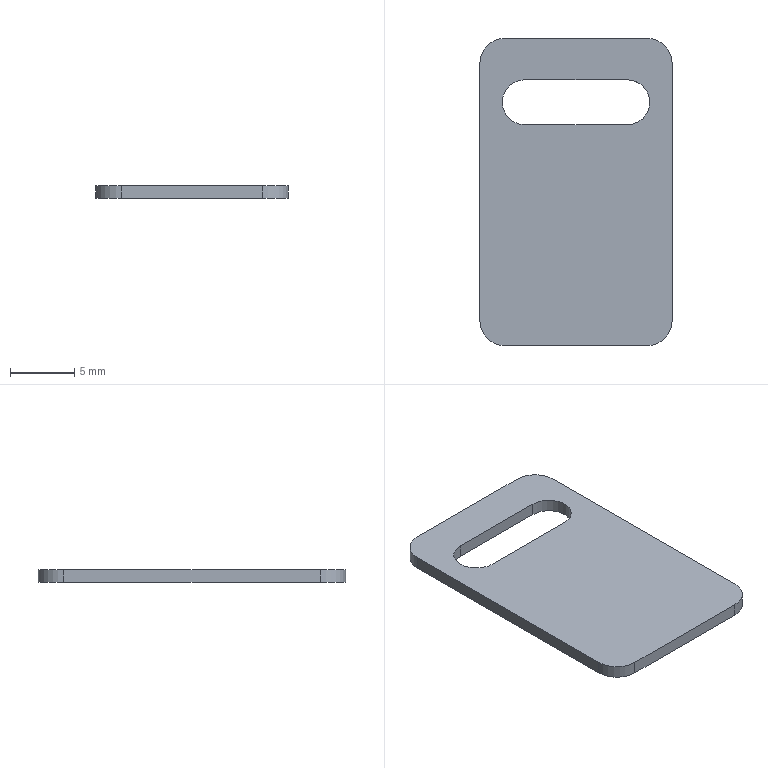Part | SolidWorks | features Extrusion 1, Fillet 1 | 1 solid | 15 faces | box 15 x 24 x 1 mm | volume 318.945 mm3 | plane 8 | cylinder 7 | commonest cylinder face diameters 4 x4 3.5 x3
STEP:
#1=CARTESIAN_POINT('',(-4.,8.75,1.));
#2=VERTEX_POINT('',#1);
#3=CARTESIAN_POINT('',(-5.75,7.,1.));
#4=VERTEX_POINT('',#3);
#5=CARTESIAN_POINT('',(-4.,7.,1.));
#6=DIRECTION('',(0.,0.,1.));
#7=DIRECTION('',(1.,0.,0.));
#8=AXIS2_PLACEMENT_3D('',#5,#6,#7);
#9=CIRCLE('',#8,1.75);
#10=EDGE_CURVE('',#2,#4,#9,.T.);
#11=ORIENTED_EDGE('',*,*,#10,.T.);
#12=CARTESIAN_POINT('',(-5.75,7.,0.));
#13=VERTEX_POINT('',#12);
#14=CARTESIAN_POINT('',(-5.75,7.,1.));
#15=DIRECTION('',(0.,0.,-1.));
#16=VECTOR('',#15,1000.);
#17=LINE('',#14,#16);
#18=EDGE_CURVE('',#4,#13,#17,.T.);
#19=ORIENTED_EDGE('',*,*,#18,.T.);
#20=CARTESIAN_POINT('',(-4.,8.75,0.));
#21=VERTEX_POINT('',#20);
#22=CARTESIAN_POINT('',(-4.,7.,0.));
#23=DIRECTION('',(0.,0.,1.));
#24=DIRECTION('',(1.,0.,0.));
#25=AXIS2_PLACEMENT_3D('',#22,#23,#24);
#26=CIRCLE('',#25,1.75);
#27=EDGE_CURVE('',#21,#13,#26,.T.);
#28=ORIENTED_EDGE('',*,*,#27,.F.);
#29=CARTESIAN_POINT('',(-4.,8.75,1.));
#30=DIRECTION('',(0.,0.,-1.));
#31=VECTOR('',#30,1000.);
#32=LINE('',#29,#31);
#33=EDGE_CURVE('',#2,#21,#32,.T.);
#34=ORIENTED_EDGE('',*,*,#33,.F.);
#35=EDGE_LOOP('',(#11,#19,#28,#34));
#36=FACE_OUTER_BOUND('',#35,.T.);
#37=CARTESIAN_POINT('',(-4.,7.,1.));
#38=DIRECTION('',(0.,0.,-1.));
#39=DIRECTION('',(-1.,0.,0.));
#40=AXIS2_PLACEMENT_3D('',#37,#38,#39);
#41=CYLINDRICAL_SURFACE('',#40,1.75);
#42=ADVANCED_FACE('',(#36),#41,.F.);
#43=CARTESIAN_POINT('',(5.5,12.,1.));
#44=VERTEX_POINT('',#43);
#45=CARTESIAN_POINT('',(-5.5,12.,1.));
#46=VERTEX_POINT('',#45);
#47=CARTESIAN_POINT('',(-7.5,12.,1.));
#48=DIRECTION('',(-1.,0.,0.));
#49=VECTOR('',#48,1000.);
#50=LINE('',#47,#49);
#51=EDGE_CURVE('',#44,#46,#50,.T.);
#52=ORIENTED_EDGE('',*,*,#51,.T.);
#53=CARTESIAN_POINT('',(-7.5,10.,1.));
#54=VERTEX_POINT('',#53);
#55=CARTESIAN_POINT('',(-5.5,10.,1.));
#56=DIRECTION('',(0.,0.,1.));
#57=DIRECTION('',(-1.,0.,0.));
#58=AXIS2_PLACEMENT_3D('',#55,#56,#57);
#59=CIRCLE('',#58,2.);
#60=EDGE_CURVE('',#46,#54,#59,.T.);
#61=ORIENTED_EDGE('',*,*,#60,.T.);
#62=CARTESIAN_POINT('',(-7.5,-10.,1.));
#63=VERTEX_POINT('',#62);
#64=CARTESIAN_POINT('',(-7.5,-12.,1.));
#65=DIRECTION('',(0.,-1.,0.));
#66=VECTOR('',#65,1000.);
#67=LINE('',#64,#66);
#68=EDGE_CURVE('',#54,#63,#67,.T.);
#69=ORIENTED_EDGE('',*,*,#68,.T.);
#70=CARTESIAN_POINT('',(-5.5,-12.,1.));
#71=VERTEX_POINT('',#70);
#72=CARTESIAN_POINT('',(-5.5,-10.,1.));
#73=DIRECTION('',(0.,0.,1.));
#74=DIRECTION('',(-1.,0.,0.));
#75=AXIS2_PLACEMENT_3D('',#72,#73,#74);
#76=CIRCLE('',#75,2.);
#77=EDGE_CURVE('',#63,#71,#76,.T.);
#78=ORIENTED_EDGE('',*,*,#77,.T.);
#79=CARTESIAN_POINT('',(5.5,-12.,1.));
#80=VERTEX_POINT('',#79);
#81=CARTESIAN_POINT('',(-7.5,-12.,1.));
#82=DIRECTION('',(1.,0.,0.));
#83=VECTOR('',#82,1000.);
#84=LINE('',#81,#83);
#85=EDGE_CURVE('',#71,#80,#84,.T.);
#86=ORIENTED_EDGE('',*,*,#85,.T.);
#87=CARTESIAN_POINT('',(7.5,-10.,1.));
#88=VERTEX_POINT('',#87);
#89=CARTESIAN_POINT('',(5.5,-10.,1.));
#90=DIRECTION('',(0.,0.,1.));
#91=DIRECTION('',(-1.,0.,0.));
#92=AXIS2_PLACEMENT_3D('',#89,#90,#91);
#93=CIRCLE('',#92,2.);
#94=EDGE_CURVE('',#80,#88,#93,.T.);
#95=ORIENTED_EDGE('',*,*,#94,.T.);
#96=CARTESIAN_POINT('',(7.5,10.,1.));
#97=VERTEX_POINT('',#96);
#98=CARTESIAN_POINT('',(7.5,-12.,1.));
#99=DIRECTION('',(0.,1.,0.));
#100=VECTOR('',#99,1000.);
#101=LINE('',#98,#100);
#102=EDGE_CURVE('',#88,#97,#101,.T.);
#103=ORIENTED_EDGE('',*,*,#102,.T.);
#104=CARTESIAN_POINT('',(5.5,10.,1.));
#105=DIRECTION('',(0.,0.,1.));
#106=DIRECTION('',(-1.,0.,0.));
#107=AXIS2_PLACEMENT_3D('',#104,#105,#106);
#108=CIRCLE('',#107,2.);
#109=EDGE_CURVE('',#97,#44,#108,.T.);
#110=ORIENTED_EDGE('',*,*,#109,.T.);
#111=EDGE_LOOP('',(#52,#61,#69,#78,#86,#95,#103,#110));
#112=FACE_OUTER_BOUND('',#111,.T.);
#113=ORIENTED_EDGE('',*,*,#10,.F.);
#114=CARTESIAN_POINT('',(4.,8.75,1.));
#115=VERTEX_POINT('',#114);
#116=CARTESIAN_POINT('',(-4.,8.75,1.));
#117=DIRECTION('',(-1.,0.,0.));
#118=VECTOR('',#117,1000.);
#119=LINE('',#116,#118);
#120=EDGE_CURVE('',#115,#2,#119,.T.);
#121=ORIENTED_EDGE('',*,*,#120,.F.);
#122=CARTESIAN_POINT('',(4.,5.25,1.));
#123=VERTEX_POINT('',#122);
#124=CARTESIAN_POINT('',(4.,7.,1.));
#125=DIRECTION('',(0.,0.,1.));
#126=DIRECTION('',(1.,0.,0.));
#127=AXIS2_PLACEMENT_3D('',#124,#125,#126);
#128=CIRCLE('',#127,1.75);
#129=EDGE_CURVE('',#123,#115,#128,.T.);
#130=ORIENTED_EDGE('',*,*,#129,.F.);
#131=CARTESIAN_POINT('',(-4.,5.25,1.));
#132=VERTEX_POINT('',#131);
#133=CARTESIAN_POINT('',(-4.,5.25,1.));
#134=DIRECTION('',(1.,0.,0.));
#135=VECTOR('',#134,1000.);
#136=LINE('',#133,#135);
#137=EDGE_CURVE('',#132,#123,#136,.T.);
#138=ORIENTED_EDGE('',*,*,#137,.F.);
#139=CARTESIAN_POINT('',(-4.,7.,1.));
#140=DIRECTION('',(0.,0.,1.));
#141=DIRECTION('',(1.,0.,0.));
#142=AXIS2_PLACEMENT_3D('',#139,#140,#141);
#143=CIRCLE('',#142,1.75);
#144=EDGE_CURVE('',#4,#132,#143,.T.);
#145=ORIENTED_EDGE('',*,*,#144,.F.);
#146=EDGE_LOOP('',(#113,#121,#130,#138,#145));
#147=FACE_BOUND('',#146,.T.);
#148=CARTESIAN_POINT('',(0.,0.,1.));
#149=DIRECTION('',(0.,0.,-1.));
#150=DIRECTION('',(-1.,0.,0.));
#151=AXIS2_PLACEMENT_3D('',#148,#149,#150);
#152=PLANE('',#151);
#153=ADVANCED_FACE('',(#112,#147),#152,.F.);
#154=CARTESIAN_POINT('',(-7.5,10.,0.));
#155=VERTEX_POINT('',#154);
#156=CARTESIAN_POINT('',(-7.5,-10.,0.));
#157=VERTEX_POINT('',#156);
#158=CARTESIAN_POINT('',(-7.5,-12.,0.));
#159=DIRECTION('',(0.,-1.,0.));
#160=VECTOR('',#159,1000.);
#161=LINE('',#158,#160);
#162=EDGE_CURVE('',#155,#157,#161,.T.);
#163=ORIENTED_EDGE('',*,*,#162,.F.);
#164=CARTESIAN_POINT('',(-5.5,12.,0.));
#165=VERTEX_POINT('',#164);
#166=CARTESIAN_POINT('',(-5.5,10.,0.));
#167=DIRECTION('',(0.,0.,-1.));
#168=DIRECTION('',(-1.,0.,0.));
#169=AXIS2_PLACEMENT_3D('',#166,#167,#168);
#170=CIRCLE('',#169,2.);
#171=EDGE_CURVE('',#155,#165,#170,.T.);
#172=ORIENTED_EDGE('',*,*,#171,.T.);
#173=CARTESIAN_POINT('',(5.5,12.,0.));
#174=VERTEX_POINT('',#173);
#175=CARTESIAN_POINT('',(-7.5,12.,0.));
#176=DIRECTION('',(-1.,0.,0.));
#177=VECTOR('',#176,1000.);
#178=LINE('',#175,#177);
#179=EDGE_CURVE('',#174,#165,#178,.T.);
#180=ORIENTED_EDGE('',*,*,#179,.F.);
#181=CARTESIAN_POINT('',(7.5,10.,0.));
#182=VERTEX_POINT('',#181);
#183=CARTESIAN_POINT('',(5.5,10.,0.));
#184=DIRECTION('',(0.,0.,-1.));
#185=DIRECTION('',(-1.,0.,0.));
#186=AXIS2_PLACEMENT_3D('',#183,#184,#185);
#187=CIRCLE('',#186,2.);
#188=EDGE_CURVE('',#174,#182,#187,.T.);
#189=ORIENTED_EDGE('',*,*,#188,.T.);
#190=CARTESIAN_POINT('',(7.5,-10.,0.));
#191=VERTEX_POINT('',#190);
#192=CARTESIAN_POINT('',(7.5,-12.,0.));
#193=DIRECTION('',(0.,1.,0.));
#194=VECTOR('',#193,1000.);
#195=LINE('',#192,#194);
#196=EDGE_CURVE('',#191,#182,#195,.T.);
#197=ORIENTED_EDGE('',*,*,#196,.F.);
#198=CARTESIAN_POINT('',(5.5,-12.,0.));
#199=VERTEX_POINT('',#198);
#200=CARTESIAN_POINT('',(5.5,-10.,0.));
#201=DIRECTION('',(0.,0.,-1.));
#202=DIRECTION('',(-1.,0.,0.));
#203=AXIS2_PLACEMENT_3D('',#200,#201,#202);
#204=CIRCLE('',#203,2.);
#205=EDGE_CURVE('',#191,#199,#204,.T.);
#206=ORIENTED_EDGE('',*,*,#205,.T.);
#207=CARTESIAN_POINT('',(-5.5,-12.,0.));
#208=VERTEX_POINT('',#207);
#209=CARTESIAN_POINT('',(-7.5,-12.,0.));
#210=DIRECTION('',(1.,0.,0.));
#211=VECTOR('',#210,1000.);
#212=LINE('',#209,#211);
#213=EDGE_CURVE('',#208,#199,#212,.T.);
#214=ORIENTED_EDGE('',*,*,#213,.F.);
#215=CARTESIAN_POINT('',(-5.5,-10.,0.));
#216=DIRECTION('',(0.,0.,-1.));
#217=DIRECTION('',(-1.,0.,0.));
#218=AXIS2_PLACEMENT_3D('',#215,#216,#217);
#219=CIRCLE('',#218,2.);
#220=EDGE_CURVE('',#208,#157,#219,.T.);
#221=ORIENTED_EDGE('',*,*,#220,.T.);
#222=EDGE_LOOP('',(#163,#172,#180,#189,#197,#206,#214,#221));
#223=FACE_OUTER_BOUND('',#222,.T.);
#224=CARTESIAN_POINT('',(4.,8.75,0.));
#225=VERTEX_POINT('',#224);
#226=CARTESIAN_POINT('',(-4.,8.75,0.));
#227=DIRECTION('',(-1.,0.,0.));
#228=VECTOR('',#227,1000.);
#229=LINE('',#226,#228);
#230=EDGE_CURVE('',#225,#21,#229,.T.);
#231=ORIENTED_EDGE('',*,*,#230,.T.);
#232=ORIENTED_EDGE('',*,*,#27,.T.);
#233=CARTESIAN_POINT('',(-4.,5.25,0.));
#234=VERTEX_POINT('',#233);
#235=CARTESIAN_POINT('',(-4.,7.,0.));
#236=DIRECTION('',(0.,0.,1.));
#237=DIRECTION('',(1.,0.,0.));
#238=AXIS2_PLACEMENT_3D('',#235,#236,#237);
#239=CIRCLE('',#238,1.75);
#240=EDGE_CURVE('',#13,#234,#239,.T.);
#241=ORIENTED_EDGE('',*,*,#240,.T.);
#242=CARTESIAN_POINT('',(4.,5.25,0.));
#243=VERTEX_POINT('',#242);
#244=CARTESIAN_POINT('',(-4.,5.25,0.));
#245=DIRECTION('',(1.,0.,0.));
#246=VECTOR('',#245,1000.);
#247=LINE('',#244,#246);
#248=EDGE_CURVE('',#234,#243,#247,.T.);
#249=ORIENTED_EDGE('',*,*,#248,.T.);
#250=CARTESIAN_POINT('',(4.,7.,0.));
#251=DIRECTION('',(0.,0.,1.));
#252=DIRECTION('',(1.,0.,0.));
#253=AXIS2_PLACEMENT_3D('',#250,#251,#252);
#254=CIRCLE('',#253,1.75);
#255=EDGE_CURVE('',#243,#225,#254,.T.);
#256=ORIENTED_EDGE('',*,*,#255,.T.);
#257=EDGE_LOOP('',(#231,#232,#241,#249,#256));
#258=FACE_BOUND('',#257,.T.);
#259=CARTESIAN_POINT('',(0.,0.,0.));
#260=DIRECTION('',(0.,0.,-1.));
#261=DIRECTION('',(-1.,0.,0.));
#262=AXIS2_PLACEMENT_3D('',#259,#260,#261);
#263=PLANE('',#262);
#264=ADVANCED_FACE('',(#223,#258),#263,.T.);
#265=ORIENTED_EDGE('',*,*,#196,.T.);
#266=CARTESIAN_POINT('',(7.5,10.,1.));
#267=DIRECTION('',(0.,0.,1.));
#268=VECTOR('',#267,1000.);
#269=LINE('',#266,#268);
#270=EDGE_CURVE('',#182,#97,#269,.T.);
#271=ORIENTED_EDGE('',*,*,#270,.T.);
#272=ORIENTED_EDGE('',*,*,#102,.F.);
#273=CARTESIAN_POINT('',(7.5,-10.,1.));
#274=DIRECTION('',(0.,0.,-1.));
#275=VECTOR('',#274,1000.);
#276=LINE('',#273,#275);
#277=EDGE_CURVE('',#88,#191,#276,.T.);
#278=ORIENTED_EDGE('',*,*,#277,.T.);
#279=EDGE_LOOP('',(#265,#271,#272,#278));
#280=FACE_OUTER_BOUND('',#279,.T.);
#281=CARTESIAN_POINT('',(7.5,-12.,1.));
#282=DIRECTION('',(-1.,0.,0.));
#283=DIRECTION('',(0.,0.,1.));
#284=AXIS2_PLACEMENT_3D('',#281,#282,#283);
#285=PLANE('',#284);
#286=ADVANCED_FACE('',(#280),#285,.F.);
#287=ORIENTED_EDGE('',*,*,#179,.T.);
#288=CARTESIAN_POINT('',(-5.5,12.,1.));
#289=DIRECTION('',(0.,0.,1.));
#290=VECTOR('',#289,1000.);
#291=LINE('',#288,#290);
#292=EDGE_CURVE('',#165,#46,#291,.T.);
#293=ORIENTED_EDGE('',*,*,#292,.T.);
#294=ORIENTED_EDGE('',*,*,#51,.F.);
#295=CARTESIAN_POINT('',(5.5,12.,1.));
#296=DIRECTION('',(0.,0.,-1.));
#297=VECTOR('',#296,1000.);
#298=LINE('',#295,#297);
#299=EDGE_CURVE('',#44,#174,#298,.T.);
#300=ORIENTED_EDGE('',*,*,#299,.T.);
#301=EDGE_LOOP('',(#287,#293,#294,#300));
#302=FACE_OUTER_BOUND('',#301,.T.);
#303=CARTESIAN_POINT('',(-7.5,12.,1.));
#304=DIRECTION('',(0.,-1.,0.));
#305=DIRECTION('',(0.,0.,-1.));
#306=AXIS2_PLACEMENT_3D('',#303,#304,#305);
#307=PLANE('',#306);
#308=ADVANCED_FACE('',(#302),#307,.F.);
#309=ORIENTED_EDGE('',*,*,#68,.F.);
#310=CARTESIAN_POINT('',(-7.5,10.,1.));
#311=DIRECTION('',(0.,0.,-1.));
#312=VECTOR('',#311,1000.);
#313=LINE('',#310,#312);
#314=EDGE_CURVE('',#54,#155,#313,.T.);
#315=ORIENTED_EDGE('',*,*,#314,.T.);
#316=ORIENTED_EDGE('',*,*,#162,.T.);
#317=CARTESIAN_POINT('',(-7.5,-10.,1.));
#318=DIRECTION('',(0.,0.,1.));
#319=VECTOR('',#318,1000.);
#320=LINE('',#317,#319);
#321=EDGE_CURVE('',#157,#63,#320,.T.);
#322=ORIENTED_EDGE('',*,*,#321,.T.);
#323=EDGE_LOOP('',(#309,#315,#316,#322));
#324=FACE_OUTER_BOUND('',#323,.T.);
#325=CARTESIAN_POINT('',(-7.5,-12.,1.));
#326=DIRECTION('',(1.,0.,0.));
#327=DIRECTION('',(0.,0.,-1.));
#328=AXIS2_PLACEMENT_3D('',#325,#326,#327);
#329=PLANE('',#328);
#330=ADVANCED_FACE('',(#324),#329,.F.);
#331=ORIENTED_EDGE('',*,*,#213,.T.);
#332=CARTESIAN_POINT('',(5.5,-12.,1.));
#333=DIRECTION('',(0.,0.,1.));
#334=VECTOR('',#333,1000.);
#335=LINE('',#332,#334);
#336=EDGE_CURVE('',#199,#80,#335,.T.);
#337=ORIENTED_EDGE('',*,*,#336,.T.);
#338=ORIENTED_EDGE('',*,*,#85,.F.);
#339=CARTESIAN_POINT('',(-5.5,-12.,1.));
#340=DIRECTION('',(0.,0.,-1.));
#341=VECTOR('',#340,1000.);
#342=LINE('',#339,#341);
#343=EDGE_CURVE('',#71,#208,#342,.T.);
#344=ORIENTED_EDGE('',*,*,#343,.T.);
#345=EDGE_LOOP('',(#331,#337,#338,#344));
#346=FACE_OUTER_BOUND('',#345,.T.);
#347=CARTESIAN_POINT('',(-7.5,-12.,1.));
#348=DIRECTION('',(0.,1.,0.));
#349=DIRECTION('',(0.,0.,1.));
#350=AXIS2_PLACEMENT_3D('',#347,#348,#349);
#351=PLANE('',#350);
#352=ADVANCED_FACE('',(#346),#351,.F.);
#353=ORIENTED_EDGE('',*,*,#18,.F.);
#354=ORIENTED_EDGE('',*,*,#144,.T.);
#355=CARTESIAN_POINT('',(-4.,5.25,1.));
#356=DIRECTION('',(0.,0.,-1.));
#357=VECTOR('',#356,1000.);
#358=LINE('',#355,#357);
#359=EDGE_CURVE('',#132,#234,#358,.T.);
#360=ORIENTED_EDGE('',*,*,#359,.T.);
#361=ORIENTED_EDGE('',*,*,#240,.F.);
#362=EDGE_LOOP('',(#353,#354,#360,#361));
#363=FACE_OUTER_BOUND('',#362,.T.);
#364=CARTESIAN_POINT('',(-4.,7.,1.));
#365=DIRECTION('',(0.,0.,-1.));
#366=DIRECTION('',(-1.,0.,0.));
#367=AXIS2_PLACEMENT_3D('',#364,#365,#366);
#368=CYLINDRICAL_SURFACE('',#367,1.75);
#369=ADVANCED_FACE('',(#363),#368,.F.);
#370=ORIENTED_EDGE('',*,*,#248,.F.);
#371=ORIENTED_EDGE('',*,*,#359,.F.);
#372=ORIENTED_EDGE('',*,*,#137,.T.);
#373=CARTESIAN_POINT('',(4.,5.25,1.));
#374=DIRECTION('',(0.,0.,-1.));
#375=VECTOR('',#374,1000.);
#376=LINE('',#373,#375);
#377=EDGE_CURVE('',#123,#243,#376,.T.);
#378=ORIENTED_EDGE('',*,*,#377,.T.);
#379=EDGE_LOOP('',(#370,#371,#372,#378));
#380=FACE_OUTER_BOUND('',#379,.T.);
#381=CARTESIAN_POINT('',(-4.,5.25,1.));
#382=DIRECTION('',(0.,1.,0.));
#383=DIRECTION('',(0.,0.,1.));
#384=AXIS2_PLACEMENT_3D('',#381,#382,#383);
#385=PLANE('',#384);
#386=ADVANCED_FACE('',(#380),#385,.T.);
#387=ORIENTED_EDGE('',*,*,#255,.F.);
#388=ORIENTED_EDGE('',*,*,#377,.F.);
#389=ORIENTED_EDGE('',*,*,#129,.T.);
#390=CARTESIAN_POINT('',(4.,8.75,1.));
#391=DIRECTION('',(0.,0.,-1.));
#392=VECTOR('',#391,1000.);
#393=LINE('',#390,#392);
#394=EDGE_CURVE('',#115,#225,#393,.T.);
#395=ORIENTED_EDGE('',*,*,#394,.T.);
#396=EDGE_LOOP('',(#387,#388,#389,#395));
#397=FACE_OUTER_BOUND('',#396,.T.);
#398=CARTESIAN_POINT('',(4.,7.,1.));
#399=DIRECTION('',(0.,0.,-1.));
#400=DIRECTION('',(-1.,0.,0.));
#401=AXIS2_PLACEMENT_3D('',#398,#399,#400);
#402=CYLINDRICAL_SURFACE('',#401,1.75);
#403=ADVANCED_FACE('',(#397),#402,.F.);
#404=ORIENTED_EDGE('',*,*,#230,.F.);
#405=ORIENTED_EDGE('',*,*,#394,.F.);
#406=ORIENTED_EDGE('',*,*,#120,.T.);
#407=ORIENTED_EDGE('',*,*,#33,.T.);
#408=EDGE_LOOP('',(#404,#405,#406,#407));
#409=FACE_OUTER_BOUND('',#408,.T.);
#410=CARTESIAN_POINT('',(-4.,8.75,1.));
#411=DIRECTION('',(0.,-1.,0.));
#412=DIRECTION('',(1.,0.,0.));
#413=AXIS2_PLACEMENT_3D('',#410,#411,#412);
#414=PLANE('',#413);
#415=ADVANCED_FACE('',(#409),#414,.T.);
#416=ORIENTED_EDGE('',*,*,#60,.F.);
#417=ORIENTED_EDGE('',*,*,#292,.F.);
#418=ORIENTED_EDGE('',*,*,#171,.F.);
#419=ORIENTED_EDGE('',*,*,#314,.F.);
#420=EDGE_LOOP('',(#416,#417,#418,#419));
#421=FACE_OUTER_BOUND('',#420,.T.);
#422=CARTESIAN_POINT('',(-5.5,10.,1.));
#423=DIRECTION('',(0.,0.,-1.));
#424=DIRECTION('',(-1.,0.,0.));
#425=AXIS2_PLACEMENT_3D('',#422,#423,#424);
#426=CYLINDRICAL_SURFACE('',#425,2.);
#427=ADVANCED_FACE('',(#421),#426,.T.);
#428=ORIENTED_EDGE('',*,*,#109,.F.);
#429=ORIENTED_EDGE('',*,*,#270,.F.);
#430=ORIENTED_EDGE('',*,*,#188,.F.);
#431=ORIENTED_EDGE('',*,*,#299,.F.);
#432=EDGE_LOOP('',(#428,#429,#430,#431));
#433=FACE_OUTER_BOUND('',#432,.T.);
#434=CARTESIAN_POINT('',(5.5,10.,1.));
#435=DIRECTION('',(0.,0.,-1.));
#436=DIRECTION('',(-1.,0.,0.));
#437=AXIS2_PLACEMENT_3D('',#434,#435,#436);
#438=CYLINDRICAL_SURFACE('',#437,2.);
#439=ADVANCED_FACE('',(#433),#438,.T.);
#440=ORIENTED_EDGE('',*,*,#94,.F.);
#441=ORIENTED_EDGE('',*,*,#336,.F.);
#442=ORIENTED_EDGE('',*,*,#205,.F.);
#443=ORIENTED_EDGE('',*,*,#277,.F.);
#444=EDGE_LOOP('',(#440,#441,#442,#443));
#445=FACE_OUTER_BOUND('',#444,.T.);
#446=CARTESIAN_POINT('',(5.5,-10.,1.));
#447=DIRECTION('',(0.,0.,-1.));
#448=DIRECTION('',(-1.,0.,0.));
#449=AXIS2_PLACEMENT_3D('',#446,#447,#448);
#450=CYLINDRICAL_SURFACE('',#449,2.);
#451=ADVANCED_FACE('',(#445),#450,.T.);
#452=ORIENTED_EDGE('',*,*,#77,.F.);
#453=ORIENTED_EDGE('',*,*,#321,.F.);
#454=ORIENTED_EDGE('',*,*,#220,.F.);
#455=ORIENTED_EDGE('',*,*,#343,.F.);
#456=EDGE_LOOP('',(#452,#453,#454,#455));
#457=FACE_OUTER_BOUND('',#456,.T.);
#458=CARTESIAN_POINT('',(-5.5,-10.,1.));
#459=DIRECTION('',(0.,0.,-1.));
#460=DIRECTION('',(-1.,0.,0.));
#461=AXIS2_PLACEMENT_3D('',#458,#459,#460);
#462=CYLINDRICAL_SURFACE('',#461,2.);
#463=ADVANCED_FACE('',(#457),#462,.T.);
#464=CLOSED_SHELL('',(#42,#153,#264,#286,#308,#330,#352,#369,#386,#403,#415,#427,#439,#451,#463));
#465=MANIFOLD_SOLID_BREP('',#464);
#466=CARTESIAN_POINT('',(0.,0.,0.));
#467=DIRECTION('',(0.,0.,1.));
#468=DIRECTION('',(1.,0.,0.));
#469=AXIS2_PLACEMENT_3D('',#466,#467,#468);
#470=(LENGTH_UNIT()NAMED_UNIT(*)SI_UNIT(.MILLI.,.METRE.));
#471=UNCERTAINTY_MEASURE_WITH_UNIT(LENGTH_MEASURE(0.00001),#470,'','');
#472=(NAMED_UNIT(*)PLANE_ANGLE_UNIT()SI_UNIT($,.RADIAN.));
#473=(NAMED_UNIT(*)SI_UNIT($,.STERADIAN.)SOLID_ANGLE_UNIT());
#474=(GEOMETRIC_REPRESENTATION_CONTEXT(3)GLOBAL_UNCERTAINTY_ASSIGNED_CONTEXT((#471))GLOBAL_UNIT_ASSIGNED_CONTEXT((#470,#472,#473))REPRESENTATION_CONTEXT('',''));
#475=ADVANCED_BREP_SHAPE_REPRESENTATION('',(#465,#469),#474);